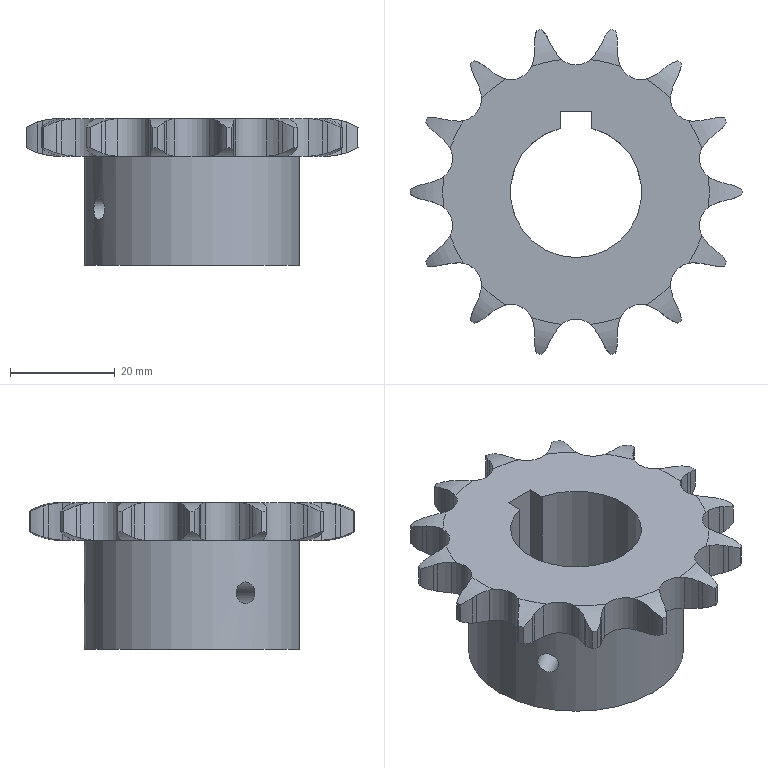Part | STEP file | 08b1-14 | 1 solid | 150 faces | box 63.262 x 61.879 x 28 mm | volume 29059 mm3 | cylinder 88 | plane 34 | torus 28 | commonest cylinder face diameters 14.27 x28 22.211 x28 8.595 x14 63.262 x14 4.134 x2 25 x1